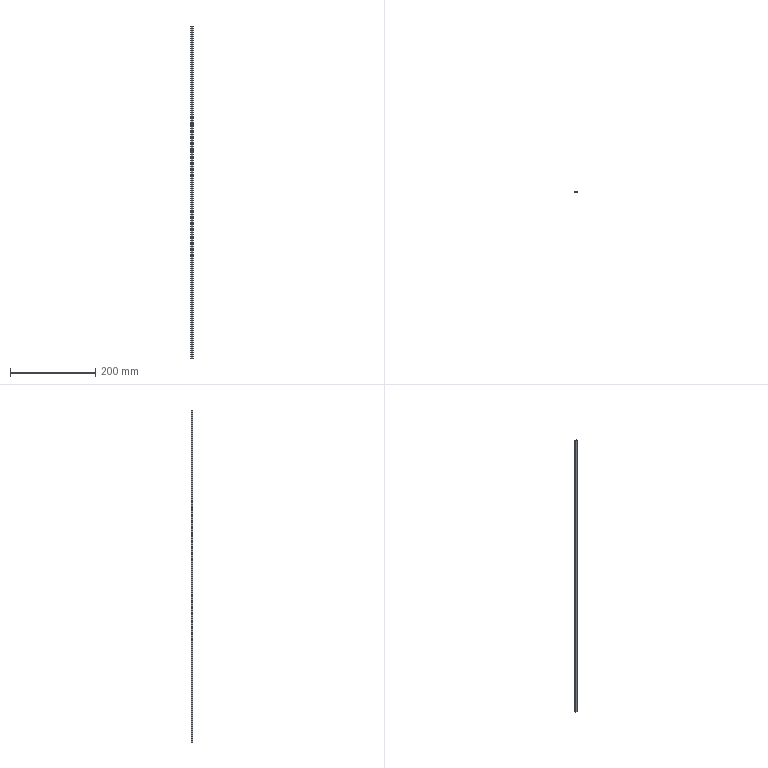Part | STEP file | BODY3_E-RAM6-S-640-ME30-C5 | 1 solid | 12 faces | box 5 x 3 x 780 mm | volume 9747 mm3 | plane 9 | cylinder 3 | commonest cylinder face diameters 0.4 x2 3.18 x1
STEP:
#1=CARTESIAN_POINT('',(-2.5,3.,-390.));
#2=VERTEX_POINT('',#1);
#3=CARTESIAN_POINT('',(-2.5,0.3,-390.));
#4=VERTEX_POINT('',#3);
#5=CARTESIAN_POINT('',(-2.5,0.,-390.));
#6=DIRECTION('',(0.,-1.,0.));
#7=VECTOR('',#6,1000.);
#8=LINE('',#5,#7);
#9=EDGE_CURVE('',#2,#4,#8,.T.);
#10=ORIENTED_EDGE('',*,*,#9,.T.);
#11=CARTESIAN_POINT('',(-2.5,0.3,390.));
#12=VERTEX_POINT('',#11);
#13=CARTESIAN_POINT('',(-2.5,0.3,390.));
#14=DIRECTION('',(0.,0.,1.));
#15=VECTOR('',#14,1000.);
#16=LINE('',#13,#15);
#17=EDGE_CURVE('',#4,#12,#16,.T.);
#18=ORIENTED_EDGE('',*,*,#17,.T.);
#19=CARTESIAN_POINT('',(-2.5,3.,390.));
#20=VERTEX_POINT('',#19);
#21=CARTESIAN_POINT('',(-2.5,0.,390.));
#22=DIRECTION('',(0.,-1.,0.));
#23=VECTOR('',#22,1000.);
#24=LINE('',#21,#23);
#25=EDGE_CURVE('',#20,#12,#24,.T.);
#26=ORIENTED_EDGE('',*,*,#25,.F.);
#27=CARTESIAN_POINT('',(-2.5,3.,390.));
#28=DIRECTION('',(0.,0.,-1.));
#29=VECTOR('',#28,1000.);
#30=LINE('',#27,#29);
#31=EDGE_CURVE('',#20,#2,#30,.T.);
#32=ORIENTED_EDGE('',*,*,#31,.T.);
#33=EDGE_LOOP('',(#10,#18,#26,#32));
#34=FACE_OUTER_BOUND('',#33,.T.);
#35=CARTESIAN_POINT('',(-2.5,0.,390.));
#36=DIRECTION('',(1.,0.,0.));
#37=DIRECTION('',(0.,0.,-1.));
#38=AXIS2_PLACEMENT_3D('',#35,#36,#37);
#39=PLANE('',#38);
#40=ADVANCED_FACE('',(#34),#39,.F.);
#41=CARTESIAN_POINT('',(-2.2,0.,390.));
#42=VERTEX_POINT('',#41);
#43=CARTESIAN_POINT('',(2.2,0.,390.));
#44=VERTEX_POINT('',#43);
#45=CARTESIAN_POINT('',(-2.5,0.,390.));
#46=DIRECTION('',(1.,0.,0.));
#47=VECTOR('',#46,1000.);
#48=LINE('',#45,#47);
#49=EDGE_CURVE('',#42,#44,#48,.T.);
#50=ORIENTED_EDGE('',*,*,#49,.F.);
#51=CARTESIAN_POINT('',(-2.2,0.,-390.));
#52=VERTEX_POINT('',#51);
#53=CARTESIAN_POINT('',(-2.2,0.,390.));
#54=DIRECTION('',(0.,0.,-1.));
#55=VECTOR('',#54,1000.);
#56=LINE('',#53,#55);
#57=EDGE_CURVE('',#42,#52,#56,.T.);
#58=ORIENTED_EDGE('',*,*,#57,.T.);
#59=CARTESIAN_POINT('',(2.2,0.,-390.));
#60=VERTEX_POINT('',#59);
#61=CARTESIAN_POINT('',(-2.5,0.,-390.));
#62=DIRECTION('',(1.,0.,0.));
#63=VECTOR('',#62,1000.);
#64=LINE('',#61,#63);
#65=EDGE_CURVE('',#52,#60,#64,.T.);
#66=ORIENTED_EDGE('',*,*,#65,.T.);
#67=CARTESIAN_POINT('',(2.2,0.,390.));
#68=DIRECTION('',(0.,0.,1.));
#69=VECTOR('',#68,1000.);
#70=LINE('',#67,#69);
#71=EDGE_CURVE('',#60,#44,#70,.T.);
#72=ORIENTED_EDGE('',*,*,#71,.T.);
#73=EDGE_LOOP('',(#50,#58,#66,#72));
#74=FACE_OUTER_BOUND('',#73,.T.);
#75=CARTESIAN_POINT('',(-2.5,0.,390.));
#76=DIRECTION('',(0.,1.,0.));
#77=DIRECTION('',(0.,0.,1.));
#78=AXIS2_PLACEMENT_3D('',#75,#76,#77);
#79=PLANE('',#78);
#80=ADVANCED_FACE('',(#74),#79,.F.);
#81=CARTESIAN_POINT('',(2.5,0.3,390.));
#82=VERTEX_POINT('',#81);
#83=CARTESIAN_POINT('',(2.5,3.,390.));
#84=VERTEX_POINT('',#83);
#85=CARTESIAN_POINT('',(2.5,0.,390.));
#86=DIRECTION('',(0.,1.,0.));
#87=VECTOR('',#86,1000.);
#88=LINE('',#85,#87);
#89=EDGE_CURVE('',#82,#84,#88,.T.);
#90=ORIENTED_EDGE('',*,*,#89,.F.);
#91=CARTESIAN_POINT('',(2.5,0.3,-390.));
#92=VERTEX_POINT('',#91);
#93=CARTESIAN_POINT('',(2.5,0.3,390.));
#94=DIRECTION('',(0.,0.,-1.));
#95=VECTOR('',#94,1000.);
#96=LINE('',#93,#95);
#97=EDGE_CURVE('',#82,#92,#96,.T.);
#98=ORIENTED_EDGE('',*,*,#97,.T.);
#99=CARTESIAN_POINT('',(2.5,3.,-390.));
#100=VERTEX_POINT('',#99);
#101=CARTESIAN_POINT('',(2.5,0.,-390.));
#102=DIRECTION('',(0.,1.,0.));
#103=VECTOR('',#102,1000.);
#104=LINE('',#101,#103);
#105=EDGE_CURVE('',#92,#100,#104,.T.);
#106=ORIENTED_EDGE('',*,*,#105,.T.);
#107=CARTESIAN_POINT('',(2.5,3.,390.));
#108=DIRECTION('',(0.,0.,-1.));
#109=VECTOR('',#108,1000.);
#110=LINE('',#107,#109);
#111=EDGE_CURVE('',#84,#100,#110,.T.);
#112=ORIENTED_EDGE('',*,*,#111,.F.);
#113=EDGE_LOOP('',(#90,#98,#106,#112));
#114=FACE_OUTER_BOUND('',#113,.T.);
#115=CARTESIAN_POINT('',(2.5,0.,390.));
#116=DIRECTION('',(-1.,0.,0.));
#117=DIRECTION('',(0.,0.,1.));
#118=AXIS2_PLACEMENT_3D('',#115,#116,#117);
#119=PLANE('',#118);
#120=ADVANCED_FACE('',(#114),#119,.F.);
#121=CARTESIAN_POINT('',(1.647,3.,-390.));
#122=VERTEX_POINT('',#121);
#123=CARTESIAN_POINT('',(1.509,3.,-390.));
#124=DIRECTION('',(-1.,0.,0.));
#125=VECTOR('',#124,1000.);
#126=LINE('',#123,#125);
#127=EDGE_CURVE('',#100,#122,#126,.T.);
#128=ORIENTED_EDGE('',*,*,#127,.T.);
#129=CARTESIAN_POINT('',(1.647,3.,390.));
#130=VERTEX_POINT('',#129);
#131=CARTESIAN_POINT('',(1.647,3.,390.));
#132=DIRECTION('',(0.,0.,1.));
#133=VECTOR('',#132,1000.);
#134=LINE('',#131,#133);
#135=EDGE_CURVE('',#122,#130,#134,.T.);
#136=ORIENTED_EDGE('',*,*,#135,.T.);
#137=CARTESIAN_POINT('',(1.509,3.,390.));
#138=DIRECTION('',(-1.,0.,0.));
#139=VECTOR('',#138,1000.);
#140=LINE('',#137,#139);
#141=EDGE_CURVE('',#84,#130,#140,.T.);
#142=ORIENTED_EDGE('',*,*,#141,.F.);
#143=ORIENTED_EDGE('',*,*,#111,.T.);
#144=EDGE_LOOP('',(#128,#136,#142,#143));
#145=FACE_OUTER_BOUND('',#144,.T.);
#146=CARTESIAN_POINT('',(1.509,3.,390.));
#147=DIRECTION('',(0.,-1.,0.));
#148=DIRECTION('',(1.,0.,0.));
#149=AXIS2_PLACEMENT_3D('',#146,#147,#148);
#150=PLANE('',#149);
#151=ADVANCED_FACE('',(#145),#150,.F.);
#152=CARTESIAN_POINT('',(1.463,2.878,390.));
#153=VERTEX_POINT('',#152);
#154=CARTESIAN_POINT('',(-1.463,2.878,390.));
#155=VERTEX_POINT('',#154);
#156=CARTESIAN_POINT('',(0.,3.5,390.));
#157=DIRECTION('',(0.,0.,-1.));
#158=DIRECTION('',(1.,0.,0.));
#159=AXIS2_PLACEMENT_3D('',#156,#157,#158);
#160=CIRCLE('',#159,1.59);
#161=EDGE_CURVE('',#153,#155,#160,.T.);
#162=ORIENTED_EDGE('',*,*,#161,.F.);
#163=CARTESIAN_POINT('',(1.463,2.878,-390.));
#164=VERTEX_POINT('',#163);
#165=CARTESIAN_POINT('',(1.463,2.878,390.));
#166=DIRECTION('',(0.,0.,-1.));
#167=VECTOR('',#166,1000.);
#168=LINE('',#165,#167);
#169=EDGE_CURVE('',#153,#164,#168,.T.);
#170=ORIENTED_EDGE('',*,*,#169,.T.);
#171=CARTESIAN_POINT('',(-1.463,2.878,-390.));
#172=VERTEX_POINT('',#171);
#173=CARTESIAN_POINT('',(0.,3.5,-390.));
#174=DIRECTION('',(0.,0.,-1.));
#175=DIRECTION('',(1.,0.,0.));
#176=AXIS2_PLACEMENT_3D('',#173,#174,#175);
#177=CIRCLE('',#176,1.59);
#178=EDGE_CURVE('',#164,#172,#177,.T.);
#179=ORIENTED_EDGE('',*,*,#178,.T.);
#180=CARTESIAN_POINT('',(-1.463,2.878,390.));
#181=DIRECTION('',(0.,0.,1.));
#182=VECTOR('',#181,1000.);
#183=LINE('',#180,#182);
#184=EDGE_CURVE('',#172,#155,#183,.T.);
#185=ORIENTED_EDGE('',*,*,#184,.T.);
#186=EDGE_LOOP('',(#162,#170,#179,#185));
#187=FACE_OUTER_BOUND('',#186,.T.);
#188=CARTESIAN_POINT('',(0.,3.5,390.));
#189=DIRECTION('',(0.,0.,-1.));
#190=DIRECTION('',(-1.,0.,0.));
#191=AXIS2_PLACEMENT_3D('',#188,#189,#190);
#192=CYLINDRICAL_SURFACE('',#191,1.59);
#193=ADVANCED_FACE('',(#187),#192,.F.);
#194=CARTESIAN_POINT('',(-1.647,3.,390.));
#195=VERTEX_POINT('',#194);
#196=CARTESIAN_POINT('',(-1.509,3.,390.));
#197=DIRECTION('',(-1.,0.,0.));
#198=VECTOR('',#197,1000.);
#199=LINE('',#196,#198);
#200=EDGE_CURVE('',#195,#20,#199,.T.);
#201=ORIENTED_EDGE('',*,*,#200,.F.);
#202=CARTESIAN_POINT('',(-1.647,3.,-390.));
#203=VERTEX_POINT('',#202);
#204=CARTESIAN_POINT('',(-1.647,3.,390.));
#205=DIRECTION('',(0.,0.,-1.));
#206=VECTOR('',#205,1000.);
#207=LINE('',#204,#206);
#208=EDGE_CURVE('',#195,#203,#207,.T.);
#209=ORIENTED_EDGE('',*,*,#208,.T.);
#210=CARTESIAN_POINT('',(-1.509,3.,-390.));
#211=DIRECTION('',(-1.,0.,0.));
#212=VECTOR('',#211,1000.);
#213=LINE('',#210,#212);
#214=EDGE_CURVE('',#203,#2,#213,.T.);
#215=ORIENTED_EDGE('',*,*,#214,.T.);
#216=ORIENTED_EDGE('',*,*,#31,.F.);
#217=EDGE_LOOP('',(#201,#209,#215,#216));
#218=FACE_OUTER_BOUND('',#217,.T.);
#219=CARTESIAN_POINT('',(-1.509,3.,390.));
#220=DIRECTION('',(0.,-1.,0.));
#221=DIRECTION('',(1.,0.,0.));
#222=AXIS2_PLACEMENT_3D('',#219,#220,#221);
#223=PLANE('',#222);
#224=ADVANCED_FACE('',(#218),#223,.F.);
#225=ORIENTED_EDGE('',*,*,#141,.T.);
#226=CARTESIAN_POINT('',(1.647,2.8,390.));
#227=DIRECTION('',(0.,0.,1.));
#228=DIRECTION('',(1.,0.,0.));
#229=AXIS2_PLACEMENT_3D('',#226,#227,#228);
#230=CIRCLE('',#229,0.2);
#231=EDGE_CURVE('',#130,#153,#230,.T.);
#232=ORIENTED_EDGE('',*,*,#231,.T.);
#233=ORIENTED_EDGE('',*,*,#161,.T.);
#234=CARTESIAN_POINT('',(-1.647,2.8,390.));
#235=DIRECTION('',(0.,0.,1.));
#236=DIRECTION('',(1.,0.,0.));
#237=AXIS2_PLACEMENT_3D('',#234,#235,#236);
#238=CIRCLE('',#237,0.2);
#239=EDGE_CURVE('',#155,#195,#238,.T.);
#240=ORIENTED_EDGE('',*,*,#239,.T.);
#241=ORIENTED_EDGE('',*,*,#200,.T.);
#242=ORIENTED_EDGE('',*,*,#25,.T.);
#243=CARTESIAN_POINT('',(-2.85,0.65,390.));
#244=DIRECTION('',(0.7071,-0.7071,0.));
#245=VECTOR('',#244,1000.);
#246=LINE('',#243,#245);
#247=EDGE_CURVE('',#12,#42,#246,.T.);
#248=ORIENTED_EDGE('',*,*,#247,.T.);
#249=ORIENTED_EDGE('',*,*,#49,.T.);
#250=CARTESIAN_POINT('',(2.85,0.65,390.));
#251=DIRECTION('',(0.7071,0.7071,0.));
#252=VECTOR('',#251,1000.);
#253=LINE('',#250,#252);
#254=EDGE_CURVE('',#44,#82,#253,.T.);
#255=ORIENTED_EDGE('',*,*,#254,.T.);
#256=ORIENTED_EDGE('',*,*,#89,.T.);
#257=EDGE_LOOP('',(#225,#232,#233,#240,#241,#242,#248,#249,#255,#256));
#258=FACE_OUTER_BOUND('',#257,.T.);
#259=CARTESIAN_POINT('',(0.,3.5,390.));
#260=DIRECTION('',(0.,0.,1.));
#261=DIRECTION('',(1.,0.,0.));
#262=AXIS2_PLACEMENT_3D('',#259,#260,#261);
#263=PLANE('',#262);
#264=ADVANCED_FACE('',(#258),#263,.T.);
#265=ORIENTED_EDGE('',*,*,#178,.F.);
#266=CARTESIAN_POINT('',(1.647,2.8,-390.));
#267=DIRECTION('',(0.,0.,-1.));
#268=DIRECTION('',(1.,0.,0.));
#269=AXIS2_PLACEMENT_3D('',#266,#267,#268);
#270=CIRCLE('',#269,0.2);
#271=EDGE_CURVE('',#164,#122,#270,.T.);
#272=ORIENTED_EDGE('',*,*,#271,.T.);
#273=ORIENTED_EDGE('',*,*,#127,.F.);
#274=ORIENTED_EDGE('',*,*,#105,.F.);
#275=CARTESIAN_POINT('',(2.5,0.3,-390.));
#276=DIRECTION('',(-0.7071,-0.7071,0.));
#277=VECTOR('',#276,1000.);
#278=LINE('',#275,#277);
#279=EDGE_CURVE('',#92,#60,#278,.T.);
#280=ORIENTED_EDGE('',*,*,#279,.T.);
#281=ORIENTED_EDGE('',*,*,#65,.F.);
#282=CARTESIAN_POINT('',(-2.2,0.,-390.));
#283=DIRECTION('',(-0.7071,0.7071,0.));
#284=VECTOR('',#283,1000.);
#285=LINE('',#282,#284);
#286=EDGE_CURVE('',#52,#4,#285,.T.);
#287=ORIENTED_EDGE('',*,*,#286,.T.);
#288=ORIENTED_EDGE('',*,*,#9,.F.);
#289=ORIENTED_EDGE('',*,*,#214,.F.);
#290=CARTESIAN_POINT('',(-1.647,2.8,-390.));
#291=DIRECTION('',(0.,0.,-1.));
#292=DIRECTION('',(1.,0.,0.));
#293=AXIS2_PLACEMENT_3D('',#290,#291,#292);
#294=CIRCLE('',#293,0.2);
#295=EDGE_CURVE('',#203,#172,#294,.T.);
#296=ORIENTED_EDGE('',*,*,#295,.T.);
#297=EDGE_LOOP('',(#265,#272,#273,#274,#280,#281,#287,#288,#289,#296));
#298=FACE_OUTER_BOUND('',#297,.T.);
#299=CARTESIAN_POINT('',(0.,3.5,-390.));
#300=DIRECTION('',(0.,0.,1.));
#301=DIRECTION('',(1.,0.,0.));
#302=AXIS2_PLACEMENT_3D('',#299,#300,#301);
#303=PLANE('',#302);
#304=ADVANCED_FACE('',(#298),#303,.F.);
#305=ORIENTED_EDGE('',*,*,#247,.F.);
#306=ORIENTED_EDGE('',*,*,#17,.F.);
#307=ORIENTED_EDGE('',*,*,#286,.F.);
#308=ORIENTED_EDGE('',*,*,#57,.F.);
#309=EDGE_LOOP('',(#305,#306,#307,#308));
#310=FACE_OUTER_BOUND('',#309,.T.);
#311=CARTESIAN_POINT('',(-2.2,0.,390.));
#312=DIRECTION('',(0.7071,0.7071,0.));
#313=DIRECTION('',(0.,0.,-1.));
#314=AXIS2_PLACEMENT_3D('',#311,#312,#313);
#315=PLANE('',#314);
#316=ADVANCED_FACE('',(#310),#315,.F.);
#317=ORIENTED_EDGE('',*,*,#254,.F.);
#318=ORIENTED_EDGE('',*,*,#71,.F.);
#319=ORIENTED_EDGE('',*,*,#279,.F.);
#320=ORIENTED_EDGE('',*,*,#97,.F.);
#321=EDGE_LOOP('',(#317,#318,#319,#320));
#322=FACE_OUTER_BOUND('',#321,.T.);
#323=CARTESIAN_POINT('',(2.5,0.3,390.));
#324=DIRECTION('',(-0.7071,0.7071,0.));
#325=DIRECTION('',(0.,0.,-1.));
#326=AXIS2_PLACEMENT_3D('',#323,#324,#325);
#327=PLANE('',#326);
#328=ADVANCED_FACE('',(#322),#327,.F.);
#329=ORIENTED_EDGE('',*,*,#231,.F.);
#330=ORIENTED_EDGE('',*,*,#135,.F.);
#331=ORIENTED_EDGE('',*,*,#271,.F.);
#332=ORIENTED_EDGE('',*,*,#169,.F.);
#333=EDGE_LOOP('',(#329,#330,#331,#332));
#334=FACE_OUTER_BOUND('',#333,.T.);
#335=CARTESIAN_POINT('',(1.647,2.8,390.));
#336=DIRECTION('',(0.,0.,-1.));
#337=DIRECTION('',(-1.,0.,0.));
#338=AXIS2_PLACEMENT_3D('',#335,#336,#337);
#339=CYLINDRICAL_SURFACE('',#338,0.2);
#340=ADVANCED_FACE('',(#334),#339,.T.);
#341=ORIENTED_EDGE('',*,*,#239,.F.);
#342=ORIENTED_EDGE('',*,*,#184,.F.);
#343=ORIENTED_EDGE('',*,*,#295,.F.);
#344=ORIENTED_EDGE('',*,*,#208,.F.);
#345=EDGE_LOOP('',(#341,#342,#343,#344));
#346=FACE_OUTER_BOUND('',#345,.T.);
#347=CARTESIAN_POINT('',(-1.647,2.8,390.));
#348=DIRECTION('',(0.,0.,-1.));
#349=DIRECTION('',(-1.,0.,0.));
#350=AXIS2_PLACEMENT_3D('',#347,#348,#349);
#351=CYLINDRICAL_SURFACE('',#350,0.2);
#352=ADVANCED_FACE('',(#346),#351,.T.);
#353=CLOSED_SHELL('',(#40,#80,#120,#151,#193,#224,#264,#304,#316,#328,#340,#352));
#354=MANIFOLD_SOLID_BREP('',#353);
#355=(LENGTH_UNIT()NAMED_UNIT(*)SI_UNIT(.MILLI.,.METRE.));
#356=UNCERTAINTY_MEASURE_WITH_UNIT(LENGTH_MEASURE(0.01),#355,'','');
#357=(NAMED_UNIT(*)PLANE_ANGLE_UNIT()SI_UNIT($,.RADIAN.));
#358=(NAMED_UNIT(*)SI_UNIT($,.STERADIAN.)SOLID_ANGLE_UNIT());
#359=(GEOMETRIC_REPRESENTATION_CONTEXT(3)GLOBAL_UNCERTAINTY_ASSIGNED_CONTEXT((#356))GLOBAL_UNIT_ASSIGNED_CONTEXT((#355,#357,#358))REPRESENTATION_CONTEXT('',''));
#360=ADVANCED_BREP_SHAPE_REPRESENTATION('',(#354),#359);